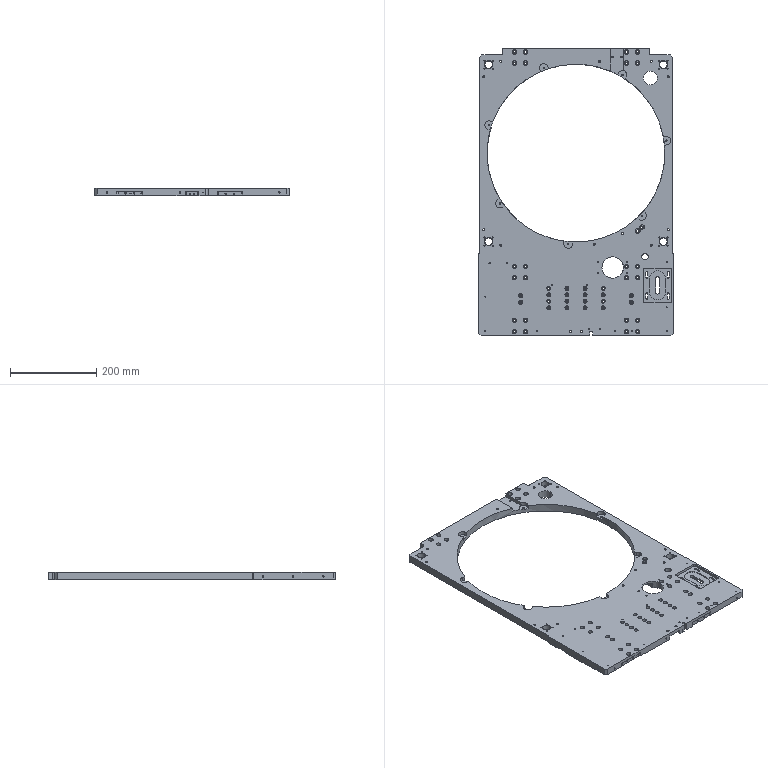Part | NX | features BREP 1 | 1 solid | 702 faces | box 450 x 665 x 18 mm | volume 2551814 mm3 | cylinder 428 | plane 211 | cone 63 | commonest cylinder face diameters 4.5 x102 3.3 x68 10 x64 2.5 x52 9 x34 5 x26